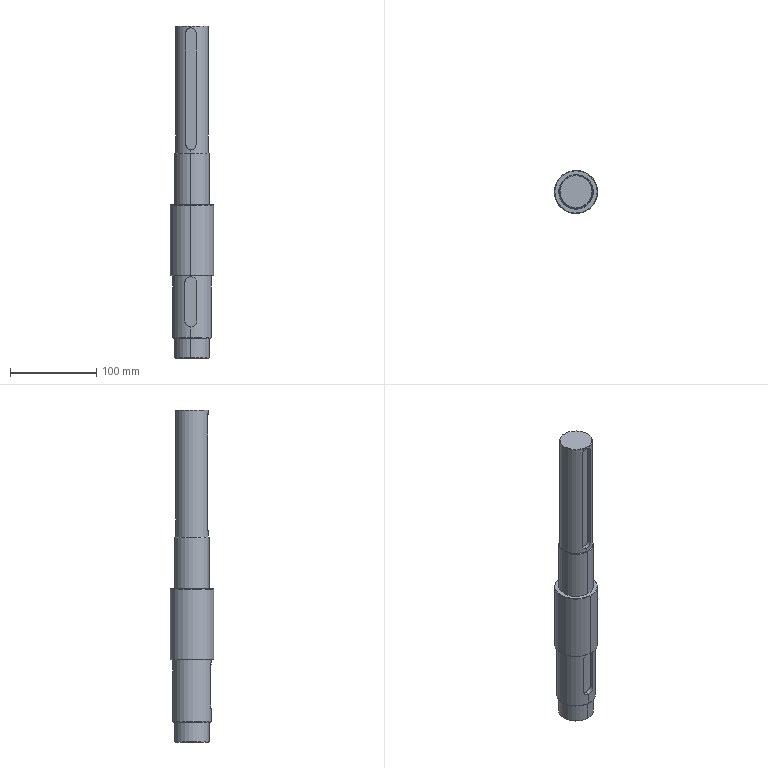Part | SolidWorks | features BaseBody 1 | 1 solid | 40 faces | box 50 x 50 x 384 mm | volume 534684 mm3 | cylinder 16 | cone 12 | plane 12 | commonest cylinder face diameters 40 x4 12 x3 14 x3 38 x2 45 x2 50 x2
STEP:
#1=CARTESIAN_POINT('',(581.983,5.282,-315.693));
#2=VERTEX_POINT('',#1);
#3=CARTESIAN_POINT('',(575.002,5.788,-322.693));
#4=VERTEX_POINT('',#3);
#5=CARTESIAN_POINT('',(575.002,5.788,-315.693));
#6=DIRECTION('',(0.07229,0.9974,0.));
#7=DIRECTION('',(0.,0.,1.));
#8=AXIS2_PLACEMENT_3D('',#5,#6,#7);
#9=CIRCLE('',#8,7.);
#10=EDGE_CURVE('',#2,#4,#9,.T.);
#11=ORIENTED_EDGE('',*,*,#10,.T.);
#12=CARTESIAN_POINT('',(574.604,0.3028,-322.693));
#13=VERTEX_POINT('',#12);
#14=CARTESIAN_POINT('',(575.002,5.788,-322.693));
#15=DIRECTION('',(-0.07229,-0.9974,0.));
#16=VECTOR('',#15,1000.);
#17=LINE('',#14,#16);
#18=EDGE_CURVE('',#4,#13,#17,.T.);
#19=ORIENTED_EDGE('',*,*,#18,.T.);
#20=CARTESIAN_POINT('',(581.667,0.9105,-315.693));
#21=VERTEX_POINT('',#20);
#22=CARTESIAN_POINT('',(574.604,0.3028,-322.693));
#23=CARTESIAN_POINT('',(575.062,0.2696,-322.693));
#24=CARTESIAN_POINT('',(575.529,0.2504,-322.647));
#25=CARTESIAN_POINT('',(576.43,0.2403,-322.466));
#26=CARTESIAN_POINT('',(576.869,0.2489,-322.333));
#27=CARTESIAN_POINT('',(577.511,0.2794,-322.068));
#28=CARTESIAN_POINT('',(577.721,0.2925,-321.969));
#29=CARTESIAN_POINT('',(578.127,0.3231,-321.753));
#30=CARTESIAN_POINT('',(578.323,0.3407,-321.635));
#31=CARTESIAN_POINT('',(578.704,0.3795,-321.383));
#32=CARTESIAN_POINT('',(578.889,0.4008,-321.247));
#33=CARTESIAN_POINT('',(579.245,0.4461,-320.958));
#34=CARTESIAN_POINT('',(579.418,0.4703,-320.803));
#35=CARTESIAN_POINT('',(579.909,0.5442,-320.319));
#36=CARTESIAN_POINT('',(580.201,0.5954,-319.969));
#37=CARTESIAN_POINT('',(580.715,0.6939,-319.214));
#38=CARTESIAN_POINT('',(580.939,0.7414,-318.805));
#39=CARTESIAN_POINT('',(581.297,0.8209,-317.963));
#40=CARTESIAN_POINT('',(581.433,0.8535,-317.527));
#41=CARTESIAN_POINT('',(581.572,0.8872,-316.849));
#42=CARTESIAN_POINT('',(581.608,0.8959,-316.619));
#43=CARTESIAN_POINT('',(581.655,0.9075,-316.157));
#44=CARTESIAN_POINT('',(581.667,0.9105,-315.926));
#45=CARTESIAN_POINT('',(581.667,0.9105,-315.693));
#46=B_SPLINE_CURVE_WITH_KNOTS('',3,(#22,#23,#24,#25,#26,#27,#28,#29,#30,#31,#32,#33,#34,#35,#36,#37,#38,#39,#40,#41,#42,#43,#44,#45),.UNSPECIFIED.,.F.,.F.,(4,2,2,2,2,2,2,2,2,2,2,4),(0.01101,0.01239,0.01376,0.01445,0.01514,0.01583,0.01651,0.01789,0.01926,0.02064,0.02133,0.02201),.UNSPECIFIED.);
#47=EDGE_CURVE('',#13,#21,#46,.T.);
#48=ORIENTED_EDGE('',*,*,#47,.T.);
#49=CARTESIAN_POINT('',(581.983,5.282,-315.693));
#50=DIRECTION('',(-0.07229,-0.9974,0.));
#51=VECTOR('',#50,1000.);
#52=LINE('',#49,#51);
#53=EDGE_CURVE('',#2,#21,#52,.T.);
#54=ORIENTED_EDGE('',*,*,#53,.F.);
#55=EDGE_LOOP('',(#11,#19,#48,#54));
#56=FACE_OUTER_BOUND('',#55,.T.);
#57=CARTESIAN_POINT('',(575.002,5.788,-315.693));
#58=DIRECTION('',(-0.07229,-0.9974,0.));
#59=DIRECTION('',(0.,0.,-1.));
#60=AXIS2_PLACEMENT_3D('',#57,#58,#59);
#61=CYLINDRICAL_SURFACE('',#60,7.);
#62=ADVANCED_FACE('',(#56),#61,.F.);
#63=CARTESIAN_POINT('',(574.893,4.292,25.307));
#64=VERTEX_POINT('',#63);
#65=CARTESIAN_POINT('',(577.568,41.196,25.307));
#66=VERTEX_POINT('',#65);
#67=CARTESIAN_POINT('',(576.231,22.744,25.307));
#68=DIRECTION('',(0.,0.,1.));
#69=DIRECTION('',(-0.07229,-0.9974,0.));
#70=AXIS2_PLACEMENT_3D('',#67,#68,#69);
#71=CIRCLE('',#70,18.5);
#72=EDGE_CURVE('',#64,#66,#71,.T.);
#73=ORIENTED_EDGE('',*,*,#72,.F.);
#74=CARTESIAN_POINT('',(574.857,3.794,24.807));
#75=VERTEX_POINT('',#74);
#76=CARTESIAN_POINT('',(574.893,4.292,25.307));
#77=DIRECTION('',(-0.05112,-0.7053,-0.7071));
#78=VECTOR('',#77,1000.);
#79=LINE('',#76,#78);
#80=EDGE_CURVE('',#64,#75,#79,.T.);
#81=ORIENTED_EDGE('',*,*,#80,.T.);
#82=CARTESIAN_POINT('',(577.604,41.694,24.807));
#83=VERTEX_POINT('',#82);
#84=CARTESIAN_POINT('',(576.231,22.744,24.807));
#85=DIRECTION('',(0.,0.,-1.));
#86=DIRECTION('',(-0.07229,-0.9974,0.));
#87=AXIS2_PLACEMENT_3D('',#84,#85,#86);
#88=CIRCLE('',#87,19.);
#89=EDGE_CURVE('',#83,#75,#88,.T.);
#90=ORIENTED_EDGE('',*,*,#89,.F.);
#91=CARTESIAN_POINT('',(577.568,41.196,25.307));
#92=DIRECTION('',(0.05112,0.7053,-0.7071));
#93=VECTOR('',#92,1000.);
#94=LINE('',#91,#93);
#95=EDGE_CURVE('',#66,#83,#94,.T.);
#96=ORIENTED_EDGE('',*,*,#95,.F.);
#97=EDGE_LOOP('',(#73,#81,#90,#96));
#98=FACE_OUTER_BOUND('',#97,.T.);
#99=CARTESIAN_POINT('',(576.231,22.744,25.307));
#100=DIRECTION('',(0.,0.,-1.));
#101=DIRECTION('',(0.07229,0.9974,0.));
#102=AXIS2_PLACEMENT_3D('',#99,#100,#101);
#103=CONICAL_SURFACE('',#102,18.5,0.7854);
#104=ADVANCED_FACE('',(#98),#103,.T.);
#105=CARTESIAN_POINT('',(577.64,42.193,-358.693));
#106=VERTEX_POINT('',#105);
#107=CARTESIAN_POINT('',(574.821,3.295,-358.693));
#108=VERTEX_POINT('',#107);
#109=CARTESIAN_POINT('',(576.231,22.744,-358.693));
#110=DIRECTION('',(0.,0.,-1.));
#111=DIRECTION('',(0.07229,0.9974,0.));
#112=AXIS2_PLACEMENT_3D('',#109,#110,#111);
#113=CIRCLE('',#112,19.5);
#114=EDGE_CURVE('',#106,#108,#113,.T.);
#115=ORIENTED_EDGE('',*,*,#114,.F.);
#116=CARTESIAN_POINT('',(577.676,42.692,-358.193));
#117=VERTEX_POINT('',#116);
#118=CARTESIAN_POINT('',(577.64,42.193,-358.693));
#119=DIRECTION('',(0.05112,0.7053,0.7071));
#120=VECTOR('',#119,1000.);
#121=LINE('',#118,#120);
#122=EDGE_CURVE('',#106,#117,#121,.T.);
#123=ORIENTED_EDGE('',*,*,#122,.T.);
#124=CARTESIAN_POINT('',(574.785,2.796,-358.193));
#125=VERTEX_POINT('',#124);
#126=CARTESIAN_POINT('',(576.231,22.744,-358.193));
#127=DIRECTION('',(0.,0.,1.));
#128=DIRECTION('',(0.07229,0.9974,0.));
#129=AXIS2_PLACEMENT_3D('',#126,#127,#128);
#130=CIRCLE('',#129,20.);
#131=EDGE_CURVE('',#125,#117,#130,.T.);
#132=ORIENTED_EDGE('',*,*,#131,.F.);
#133=CARTESIAN_POINT('',(574.821,3.295,-358.693));
#134=DIRECTION('',(-0.05112,-0.7053,0.7071));
#135=VECTOR('',#134,1000.);
#136=LINE('',#133,#135);
#137=EDGE_CURVE('',#108,#125,#136,.T.);
#138=ORIENTED_EDGE('',*,*,#137,.F.);
#139=EDGE_LOOP('',(#115,#123,#132,#138));
#140=FACE_OUTER_BOUND('',#139,.T.);
#141=CARTESIAN_POINT('',(576.231,22.744,-358.693));
#142=DIRECTION('',(0.,0.,1.));
#143=DIRECTION('',(-0.07229,-0.9974,0.));
#144=AXIS2_PLACEMENT_3D('',#141,#142,#143);
#145=CONICAL_SURFACE('',#144,19.5,0.7854);
#146=ADVANCED_FACE('',(#140),#145,.T.);
#147=CARTESIAN_POINT('',(577.821,44.686,-335.693));
#148=VERTEX_POINT('',#147);
#149=CARTESIAN_POINT('',(574.64,0.8015,-335.693));
#150=VERTEX_POINT('',#149);
#151=CARTESIAN_POINT('',(576.231,22.744,-335.693));
#152=DIRECTION('',(0.,0.,-1.));
#153=DIRECTION('',(0.07229,0.9974,0.));
#154=AXIS2_PLACEMENT_3D('',#151,#152,#153);
#155=CIRCLE('',#154,22.);
#156=EDGE_CURVE('',#148,#150,#155,.T.);
#157=ORIENTED_EDGE('',*,*,#156,.F.);
#158=CARTESIAN_POINT('',(577.857,45.185,-335.193));
#159=VERTEX_POINT('',#158);
#160=CARTESIAN_POINT('',(577.821,44.686,-335.693));
#161=DIRECTION('',(0.05112,0.7053,0.7071));
#162=VECTOR('',#161,1000.);
#163=LINE('',#160,#162);
#164=EDGE_CURVE('',#148,#159,#163,.T.);
#165=ORIENTED_EDGE('',*,*,#164,.T.);
#166=CARTESIAN_POINT('',(574.604,0.3028,-335.193));
#167=VERTEX_POINT('',#166);
#168=CARTESIAN_POINT('',(576.231,22.744,-335.193));
#169=DIRECTION('',(0.,0.,1.));
#170=DIRECTION('',(0.07229,0.9974,0.));
#171=AXIS2_PLACEMENT_3D('',#168,#169,#170);
#172=CIRCLE('',#171,22.5);
#173=EDGE_CURVE('',#167,#159,#172,.T.);
#174=ORIENTED_EDGE('',*,*,#173,.F.);
#175=CARTESIAN_POINT('',(574.64,0.8015,-335.693));
#176=DIRECTION('',(-0.05112,-0.7053,0.7071));
#177=VECTOR('',#176,1000.);
#178=LINE('',#175,#177);
#179=EDGE_CURVE('',#150,#167,#178,.T.);
#180=ORIENTED_EDGE('',*,*,#179,.F.);
#181=EDGE_LOOP('',(#157,#165,#174,#180));
#182=FACE_OUTER_BOUND('',#181,.T.);
#183=CARTESIAN_POINT('',(576.231,22.744,-335.693));
#184=DIRECTION('',(0.,0.,1.));
#185=DIRECTION('',(-0.07229,-0.9974,0.));
#186=AXIS2_PLACEMENT_3D('',#183,#184,#185);
#187=CONICAL_SURFACE('',#186,22.,0.7854);
#188=ADVANCED_FACE('',(#182),#187,.T.);
#189=CARTESIAN_POINT('',(578.002,47.18,-263.693));
#190=VERTEX_POINT('',#189);
#191=CARTESIAN_POINT('',(574.46,-1.692,-263.693));
#192=VERTEX_POINT('',#191);
#193=CARTESIAN_POINT('',(576.231,22.744,-263.693));
#194=DIRECTION('',(0.,0.,-1.));
#195=DIRECTION('',(0.07229,0.9974,0.));
#196=AXIS2_PLACEMENT_3D('',#193,#194,#195);
#197=CIRCLE('',#196,24.5);
#198=EDGE_CURVE('',#190,#192,#197,.T.);
#199=ORIENTED_EDGE('',*,*,#198,.F.);
#200=CARTESIAN_POINT('',(578.038,47.679,-263.193));
#201=VERTEX_POINT('',#200);
#202=CARTESIAN_POINT('',(578.002,47.18,-263.693));
#203=DIRECTION('',(0.05112,0.7053,0.7071));
#204=VECTOR('',#203,1000.);
#205=LINE('',#202,#204);
#206=EDGE_CURVE('',#190,#201,#205,.T.);
#207=ORIENTED_EDGE('',*,*,#206,.T.);
#208=CARTESIAN_POINT('',(574.423,-2.191,-263.193));
#209=VERTEX_POINT('',#208);
#210=CARTESIAN_POINT('',(576.231,22.744,-263.193));
#211=DIRECTION('',(0.,0.,1.));
#212=DIRECTION('',(0.07229,0.9974,0.));
#213=AXIS2_PLACEMENT_3D('',#210,#211,#212);
#214=CIRCLE('',#213,25.);
#215=EDGE_CURVE('',#209,#201,#214,.T.);
#216=ORIENTED_EDGE('',*,*,#215,.F.);
#217=CARTESIAN_POINT('',(574.46,-1.692,-263.693));
#218=DIRECTION('',(-0.05112,-0.7053,0.7071));
#219=VECTOR('',#218,1000.);
#220=LINE('',#217,#219);
#221=EDGE_CURVE('',#192,#209,#220,.T.);
#222=ORIENTED_EDGE('',*,*,#221,.F.);
#223=EDGE_LOOP('',(#199,#207,#216,#222));
#224=FACE_OUTER_BOUND('',#223,.T.);
#225=CARTESIAN_POINT('',(576.231,22.744,-263.693));
#226=DIRECTION('',(0.,0.,1.));
#227=DIRECTION('',(-0.07229,-0.9974,0.));
#228=AXIS2_PLACEMENT_3D('',#225,#226,#227);
#229=CONICAL_SURFACE('',#228,24.5,0.7854);
#230=ADVANCED_FACE('',(#224),#229,.T.);
#231=CARTESIAN_POINT('',(574.821,3.295,-121.693));
#232=VERTEX_POINT('',#231);
#233=CARTESIAN_POINT('',(577.64,42.193,-121.693));
#234=VERTEX_POINT('',#233);
#235=CARTESIAN_POINT('',(576.231,22.744,-121.693));
#236=DIRECTION('',(0.,0.,1.));
#237=DIRECTION('',(-0.07229,-0.9974,0.));
#238=AXIS2_PLACEMENT_3D('',#235,#236,#237);
#239=CIRCLE('',#238,19.5);
#240=EDGE_CURVE('',#232,#234,#239,.T.);
#241=ORIENTED_EDGE('',*,*,#240,.F.);
#242=CARTESIAN_POINT('',(574.785,2.796,-122.193));
#243=VERTEX_POINT('',#242);
#244=CARTESIAN_POINT('',(574.821,3.295,-121.693));
#245=DIRECTION('',(-0.05112,-0.7053,-0.7071));
#246=VECTOR('',#245,1000.);
#247=LINE('',#244,#246);
#248=EDGE_CURVE('',#232,#243,#247,.T.);
#249=ORIENTED_EDGE('',*,*,#248,.T.);
#250=CARTESIAN_POINT('',(577.676,42.692,-122.193));
#251=VERTEX_POINT('',#250);
#252=CARTESIAN_POINT('',(576.231,22.744,-122.193));
#253=DIRECTION('',(0.,0.,-1.));
#254=DIRECTION('',(-0.07229,-0.9974,0.));
#255=AXIS2_PLACEMENT_3D('',#252,#253,#254);
#256=CIRCLE('',#255,20.);
#257=EDGE_CURVE('',#251,#243,#256,.T.);
#258=ORIENTED_EDGE('',*,*,#257,.F.);
#259=CARTESIAN_POINT('',(577.64,42.193,-121.693));
#260=DIRECTION('',(0.05112,0.7053,-0.7071));
#261=VECTOR('',#260,1000.);
#262=LINE('',#259,#261);
#263=EDGE_CURVE('',#234,#251,#262,.T.);
#264=ORIENTED_EDGE('',*,*,#263,.F.);
#265=EDGE_LOOP('',(#241,#249,#258,#264));
#266=FACE_OUTER_BOUND('',#265,.T.);
#267=CARTESIAN_POINT('',(576.231,22.744,-121.693));
#268=DIRECTION('',(0.,0.,-1.));
#269=DIRECTION('',(0.07229,0.9974,0.));
#270=AXIS2_PLACEMENT_3D('',#267,#268,#269);
#271=CONICAL_SURFACE('',#270,19.5,0.7854);
#272=ADVANCED_FACE('',(#266),#271,.T.);
#273=CARTESIAN_POINT('',(574.46,-1.692,-181.693));
#274=VERTEX_POINT('',#273);
#275=CARTESIAN_POINT('',(578.002,47.18,-181.693));
#276=VERTEX_POINT('',#275);
#277=CARTESIAN_POINT('',(576.231,22.744,-181.693));
#278=DIRECTION('',(0.,0.,1.));
#279=DIRECTION('',(0.07229,0.9974,0.));
#280=AXIS2_PLACEMENT_3D('',#277,#278,#279);
#281=CIRCLE('',#280,24.5);
#282=EDGE_CURVE('',#274,#276,#281,.T.);
#283=ORIENTED_EDGE('',*,*,#282,.F.);
#284=CARTESIAN_POINT('',(574.423,-2.191,-182.193));
#285=VERTEX_POINT('',#284);
#286=CARTESIAN_POINT('',(574.423,-2.191,-182.193));
#287=DIRECTION('',(-0.05112,-0.7053,-0.7071));
#288=VECTOR('',#287,1000.);
#289=LINE('',#286,#288);
#290=EDGE_CURVE('',#274,#285,#289,.T.);
#291=ORIENTED_EDGE('',*,*,#290,.T.);
#292=CARTESIAN_POINT('',(578.038,47.679,-182.193));
#293=VERTEX_POINT('',#292);
#294=CARTESIAN_POINT('',(576.231,22.744,-182.193));
#295=DIRECTION('',(0.,0.,-1.));
#296=DIRECTION('',(0.07229,0.9974,0.));
#297=AXIS2_PLACEMENT_3D('',#294,#295,#296);
#298=CIRCLE('',#297,25.);
#299=EDGE_CURVE('',#293,#285,#298,.T.);
#300=ORIENTED_EDGE('',*,*,#299,.F.);
#301=CARTESIAN_POINT('',(578.038,47.679,-182.193));
#302=DIRECTION('',(0.05112,0.7053,-0.7071));
#303=VECTOR('',#302,1000.);
#304=LINE('',#301,#303);
#305=EDGE_CURVE('',#276,#293,#304,.T.);
#306=ORIENTED_EDGE('',*,*,#305,.F.);
#307=EDGE_LOOP('',(#283,#291,#300,#306));
#308=FACE_OUTER_BOUND('',#307,.T.);
#309=CARTESIAN_POINT('',(576.231,22.744,-182.193));
#310=DIRECTION('',(0.,0.,-1.));
#311=DIRECTION('',(0.07229,0.9974,0.));
#312=AXIS2_PLACEMENT_3D('',#309,#310,#311);
#313=CONICAL_SURFACE('',#312,25.,0.7854);
#314=ADVANCED_FACE('',(#308),#313,.T.);
#315=CARTESIAN_POINT('',(581.203,8.347,-111.693));
#316=VERTEX_POINT('',#315);
#317=CARTESIAN_POINT('',(575.219,8.781,-117.693));
#318=VERTEX_POINT('',#317);
#319=CARTESIAN_POINT('',(575.219,8.781,-111.693));
#320=DIRECTION('',(0.07229,0.9974,0.));
#321=DIRECTION('',(0.,0.,1.));
#322=AXIS2_PLACEMENT_3D('',#319,#320,#321);
#323=CIRCLE('',#322,6.);
#324=EDGE_CURVE('',#316,#318,#323,.T.);
#325=ORIENTED_EDGE('',*,*,#324,.T.);
#326=CARTESIAN_POINT('',(574.857,3.794,-117.693));
#327=VERTEX_POINT('',#326);
#328=CARTESIAN_POINT('',(575.219,8.781,-117.693));
#329=DIRECTION('',(-0.07229,-0.9974,0.));
#330=VECTOR('',#329,1000.);
#331=LINE('',#328,#330);
#332=EDGE_CURVE('',#318,#327,#331,.T.);
#333=ORIENTED_EDGE('',*,*,#332,.T.);
#334=CARTESIAN_POINT('',(580.912,4.33,-111.693));
#335=VERTEX_POINT('',#334);
#336=CARTESIAN_POINT('',(574.857,3.794,-117.693));
#337=CARTESIAN_POINT('',(575.25,3.765,-117.693));
#338=CARTESIAN_POINT('',(575.65,3.749,-117.653));
#339=CARTESIAN_POINT('',(576.422,3.741,-117.499));
#340=CARTESIAN_POINT('',(576.799,3.749,-117.384));
#341=CARTESIAN_POINT('',(577.533,3.785,-117.081));
#342=CARTESIAN_POINT('',(577.882,3.813,-116.895));
#343=CARTESIAN_POINT('',(578.372,3.864,-116.57));
#344=CARTESIAN_POINT('',(578.53,3.883,-116.454));
#345=CARTESIAN_POINT('',(578.836,3.923,-116.206));
#346=CARTESIAN_POINT('',(578.984,3.944,-116.073));
#347=CARTESIAN_POINT('',(579.404,4.009,-115.658));
#348=CARTESIAN_POINT('',(579.655,4.054,-115.358));
#349=CARTESIAN_POINT('',(580.096,4.14,-114.711));
#350=CARTESIAN_POINT('',(580.288,4.182,-114.361));
#351=CARTESIAN_POINT('',(580.594,4.251,-113.639));
#352=CARTESIAN_POINT('',(580.711,4.28,-113.265));
#353=CARTESIAN_POINT('',(580.871,4.319,-112.49));
#354=CARTESIAN_POINT('',(580.912,4.33,-112.092));
#355=CARTESIAN_POINT('',(580.912,4.33,-111.693));
#356=B_SPLINE_CURVE_WITH_KNOTS('',3,(#336,#337,#338,#339,#340,#341,#342,#343,#344,#345,#346,#347,#348,#349,#350,#351,#352,#353,#354,#355),.UNSPECIFIED.,.F.,.F.,(4,2,2,2,2,2,2,2,2,4),(0.009443,0.01062,0.0118,0.01298,0.01357,0.01416,0.01534,0.01652,0.01769,0.01887),.UNSPECIFIED.);
#357=EDGE_CURVE('',#327,#335,#356,.T.);
#358=ORIENTED_EDGE('',*,*,#357,.T.);
#359=CARTESIAN_POINT('',(581.203,8.347,-111.693));
#360=DIRECTION('',(-0.07229,-0.9974,0.));
#361=VECTOR('',#360,1000.);
#362=LINE('',#359,#361);
#363=EDGE_CURVE('',#316,#335,#362,.T.);
#364=ORIENTED_EDGE('',*,*,#363,.F.);
#365=EDGE_LOOP('',(#325,#333,#358,#364));
#366=FACE_OUTER_BOUND('',#365,.T.);
#367=CARTESIAN_POINT('',(575.219,8.781,-111.693));
#368=DIRECTION('',(-0.07229,-0.9974,0.));
#369=DIRECTION('',(0.,0.,-1.));
#370=AXIS2_PLACEMENT_3D('',#367,#368,#369);
#371=CYLINDRICAL_SURFACE('',#370,6.);
#372=ADVANCED_FACE('',(#366),#371,.F.);
#373=ORIENTED_EDGE('',*,*,#257,.T.);
#374=CARTESIAN_POINT('',(574.785,2.796,-181.693));
#375=VERTEX_POINT('',#374);
#376=CARTESIAN_POINT('',(574.785,2.796,-121.693));
#377=DIRECTION('',(0.,0.,-1.));
#378=VECTOR('',#377,1000.);
#379=LINE('',#376,#378);
#380=EDGE_CURVE('',#243,#375,#379,.T.);
#381=ORIENTED_EDGE('',*,*,#380,.T.);
#382=CARTESIAN_POINT('',(577.676,42.692,-181.693));
#383=VERTEX_POINT('',#382);
#384=CARTESIAN_POINT('',(576.231,22.744,-181.693));
#385=DIRECTION('',(0.,0.,1.));
#386=DIRECTION('',(0.07229,0.9974,0.));
#387=AXIS2_PLACEMENT_3D('',#384,#385,#386);
#388=CIRCLE('',#387,20.);
#389=EDGE_CURVE('',#375,#383,#388,.T.);
#390=ORIENTED_EDGE('',*,*,#389,.T.);
#391=CARTESIAN_POINT('',(577.676,42.692,-121.693));
#392=DIRECTION('',(0.,0.,-1.));
#393=VECTOR('',#392,1000.);
#394=LINE('',#391,#393);
#395=EDGE_CURVE('',#251,#383,#394,.T.);
#396=ORIENTED_EDGE('',*,*,#395,.F.);
#397=EDGE_LOOP('',(#373,#381,#390,#396));
#398=FACE_OUTER_BOUND('',#397,.T.);
#399=CARTESIAN_POINT('',(576.231,22.744,-121.693));
#400=DIRECTION('',(0.,0.,-1.));
#401=DIRECTION('',(0.07229,0.9974,0.));
#402=AXIS2_PLACEMENT_3D('',#399,#400,#401);
#403=CYLINDRICAL_SURFACE('',#402,20.);
#404=ADVANCED_FACE('',(#398),#403,.T.);
#405=ORIENTED_EDGE('',*,*,#131,.T.);
#406=CARTESIAN_POINT('',(577.676,42.692,-335.693));
#407=VERTEX_POINT('',#406);
#408=CARTESIAN_POINT('',(577.676,42.692,-358.693));
#409=DIRECTION('',(0.,0.,1.));
#410=VECTOR('',#409,1000.);
#411=LINE('',#408,#410);
#412=EDGE_CURVE('',#117,#407,#411,.T.);
#413=ORIENTED_EDGE('',*,*,#412,.T.);
#414=CARTESIAN_POINT('',(574.785,2.796,-335.693));
#415=VERTEX_POINT('',#414);
#416=CARTESIAN_POINT('',(576.231,22.744,-335.693));
#417=DIRECTION('',(0.,0.,-1.));
#418=DIRECTION('',(0.07229,0.9974,0.));
#419=AXIS2_PLACEMENT_3D('',#416,#417,#418);
#420=CIRCLE('',#419,20.);
#421=EDGE_CURVE('',#407,#415,#420,.T.);
#422=ORIENTED_EDGE('',*,*,#421,.T.);
#423=CARTESIAN_POINT('',(574.785,2.796,-358.693));
#424=DIRECTION('',(0.,0.,1.));
#425=VECTOR('',#424,1000.);
#426=LINE('',#423,#425);
#427=EDGE_CURVE('',#125,#415,#426,.T.);
#428=ORIENTED_EDGE('',*,*,#427,.F.);
#429=EDGE_LOOP('',(#405,#413,#422,#428));
#430=FACE_OUTER_BOUND('',#429,.T.);
#431=CARTESIAN_POINT('',(576.231,22.744,-358.693));
#432=DIRECTION('',(0.,0.,1.));
#433=DIRECTION('',(-0.07229,-0.9974,0.));
#434=AXIS2_PLACEMENT_3D('',#431,#432,#433);
#435=CYLINDRICAL_SURFACE('',#434,20.);
#436=ADVANCED_FACE('',(#430),#435,.T.);
#437=ORIENTED_EDGE('',*,*,#215,.T.);
#438=CARTESIAN_POINT('',(578.038,47.679,-263.693));
#439=DIRECTION('',(0.,0.,1.));
#440=VECTOR('',#439,1000.);
#441=LINE('',#438,#440);
#442=EDGE_CURVE('',#201,#293,#441,.T.);
#443=ORIENTED_EDGE('',*,*,#442,.T.);
#444=ORIENTED_EDGE('',*,*,#299,.T.);
#445=CARTESIAN_POINT('',(574.423,-2.191,-263.693));
#446=DIRECTION('',(0.,0.,1.));
#447=VECTOR('',#446,1000.);
#448=LINE('',#445,#447);
#449=EDGE_CURVE('',#209,#285,#448,.T.);
#450=ORIENTED_EDGE('',*,*,#449,.F.);
#451=EDGE_LOOP('',(#437,#443,#444,#450));
#452=FACE_OUTER_BOUND('',#451,.T.);
#453=CARTESIAN_POINT('',(576.231,22.744,-263.693));
#454=DIRECTION('',(0.,0.,1.));
#455=DIRECTION('',(-0.07229,-0.9974,0.));
#456=AXIS2_PLACEMENT_3D('',#453,#454,#455);
#457=CYLINDRICAL_SURFACE('',#456,25.);
#458=ADVANCED_FACE('',(#452),#457,.T.);
#459=ORIENTED_EDGE('',*,*,#89,.T.);
#460=CARTESIAN_POINT('',(574.857,3.794,23.307));
#461=VERTEX_POINT('',#460);
#462=CARTESIAN_POINT('',(574.857,3.794,25.307));
#463=DIRECTION('',(0.,0.,-1.));
#464=VECTOR('',#463,1000.);
#465=LINE('',#462,#464);
#466=EDGE_CURVE('',#75,#461,#465,.T.);
#467=ORIENTED_EDGE('',*,*,#466,.T.);
#468=CARTESIAN_POINT('',(580.912,4.33,17.307));
#469=VERTEX_POINT('',#468);
#470=CARTESIAN_POINT('',(580.912,4.33,17.307));
#471=CARTESIAN_POINT('',(580.912,4.33,17.706));
#472=CARTESIAN_POINT('',(580.871,4.319,18.098));
#473=CARTESIAN_POINT('',(580.753,4.29,18.676));
#474=CARTESIAN_POINT('',(580.704,4.278,18.867));
#475=CARTESIAN_POINT('',(580.587,4.25,19.246));
#476=CARTESIAN_POINT('',(580.518,4.234,19.433));
#477=CARTESIAN_POINT('',(580.287,4.181,19.977));
#478=CARTESIAN_POINT('',(580.099,4.141,20.321));
#479=CARTESIAN_POINT('',(579.767,4.076,20.808));
#480=CARTESIAN_POINT('',(579.647,4.053,20.967));
#481=CARTESIAN_POINT('',(579.394,4.009,21.27));
#482=CARTESIAN_POINT('',(579.261,3.987,21.414));
#483=CARTESIAN_POINT('',(578.843,3.922,21.826));
#484=CARTESIAN_POINT('',(578.538,3.882,22.074));
#485=CARTESIAN_POINT('',(577.876,3.812,22.513));
#486=CARTESIAN_POINT('',(577.528,3.785,22.697));
#487=CARTESIAN_POINT('',(576.983,3.758,22.922));
#488=CARTESIAN_POINT('',(576.798,3.751,22.989));
#489=CARTESIAN_POINT('',(576.419,3.744,23.104));
#490=CARTESIAN_POINT('',(576.225,3.743,23.152));
#491=CARTESIAN_POINT('',(575.642,3.749,23.269));
#492=CARTESIAN_POINT('',(575.251,3.765,23.307));
#493=CARTESIAN_POINT('',(574.857,3.794,23.307));
#494=B_SPLINE_CURVE_WITH_KNOTS('',3,(#470,#471,#472,#473,#474,#475,#476,#477,#478,#479,#480,#481,#482,#483,#484,#485,#486,#487,#488,#489,#490,#491,#492,#493),.UNSPECIFIED.,.F.,.F.,(4,2,2,2,2,2,2,2,2,2,2,4),(0.,0.00118,0.00177,0.002361,0.003541,0.004131,0.004721,0.005902,0.007082,0.007672,0.008262,0.009443),.UNSPECIFIED.);
#495=EDGE_CURVE('',#469,#461,#494,.T.);
#496=ORIENTED_EDGE('',*,*,#495,.F.);
#497=CARTESIAN_POINT('',(580.912,4.33,25.307));
#498=DIRECTION('',(0.,0.,1.));
#499=VECTOR('',#498,1000.);
#500=LINE('',#497,#499);
#501=EDGE_CURVE('',#335,#469,#500,.T.);
#502=ORIENTED_EDGE('',*,*,#501,.F.);
#503=ORIENTED_EDGE('',*,*,#357,.F.);
#504=CARTESIAN_POINT('',(574.857,3.794,-121.693));
#505=VERTEX_POINT('',#504);
#506=CARTESIAN_POINT('',(574.857,3.794,25.307));
#507=DIRECTION('',(0.,0.,-1.));
#508=VECTOR('',#507,1000.);
#509=LINE('',#506,#508);
#510=EDGE_CURVE('',#327,#505,#509,.T.);
#511=ORIENTED_EDGE('',*,*,#510,.T.);
#512=CARTESIAN_POINT('',(577.604,41.694,-121.693));
#513=VERTEX_POINT('',#512);
#514=CARTESIAN_POINT('',(576.231,22.744,-121.693));
#515=DIRECTION('',(0.,0.,1.));
#516=DIRECTION('',(-0.07229,-0.9974,0.));
#517=AXIS2_PLACEMENT_3D('',#514,#515,#516);
#518=CIRCLE('',#517,19.);
#519=EDGE_CURVE('',#505,#513,#518,.T.);
#520=ORIENTED_EDGE('',*,*,#519,.T.);
#521=CARTESIAN_POINT('',(577.604,41.694,25.307));
#522=DIRECTION('',(0.,0.,-1.));
#523=VECTOR('',#522,1000.);
#524=LINE('',#521,#523);
#525=EDGE_CURVE('',#83,#513,#524,.T.);
#526=ORIENTED_EDGE('',*,*,#525,.F.);
#527=EDGE_LOOP('',(#459,#467,#496,#502,#503,#511,#520,#526));
#528=FACE_OUTER_BOUND('',#527,.T.);
#529=CARTESIAN_POINT('',(576.231,22.744,25.307));
#530=DIRECTION('',(0.,0.,-1.));
#531=DIRECTION('',(0.07229,0.9974,0.));
#532=AXIS2_PLACEMENT_3D('',#529,#530,#531);
#533=CYLINDRICAL_SURFACE('',#532,19.);
#534=ADVANCED_FACE('',(#528),#533,.T.);
#535=ORIENTED_EDGE('',*,*,#173,.T.);
#536=CARTESIAN_POINT('',(577.857,45.185,-263.693));
#537=VERTEX_POINT('',#536);
#538=CARTESIAN_POINT('',(577.857,45.185,-335.693));
#539=DIRECTION('',(0.,0.,1.));
#540=VECTOR('',#539,1000.);
#541=LINE('',#538,#540);
#542=EDGE_CURVE('',#159,#537,#541,.T.);
#543=ORIENTED_EDGE('',*,*,#542,.T.);
#544=CARTESIAN_POINT('',(574.604,0.3028,-263.693));
#545=VERTEX_POINT('',#544);
#546=CARTESIAN_POINT('',(576.231,22.744,-263.693));
#547=DIRECTION('',(0.,0.,-1.));
#548=DIRECTION('',(0.07229,0.9974,0.));
#549=AXIS2_PLACEMENT_3D('',#546,#547,#548);
#550=CIRCLE('',#549,22.5);
#551=EDGE_CURVE('',#537,#545,#550,.T.);
#552=ORIENTED_EDGE('',*,*,#551,.T.);
#553=CARTESIAN_POINT('',(574.604,0.3028,-264.693));
#554=VERTEX_POINT('',#553);
#555=CARTESIAN_POINT('',(574.604,0.3028,-335.693));
#556=DIRECTION('',(0.,0.,1.));
#557=VECTOR('',#556,1000.);
#558=LINE('',#555,#557);
#559=EDGE_CURVE('',#554,#545,#558,.T.);
#560=ORIENTED_EDGE('',*,*,#559,.F.);
#561=CARTESIAN_POINT('',(581.667,0.9105,-271.693));
#562=VERTEX_POINT('',#561);
#563=CARTESIAN_POINT('',(581.667,0.9105,-271.693));
#564=CARTESIAN_POINT('',(581.667,0.9105,-271.227));
#565=CARTESIAN_POINT('',(581.62,0.8986,-270.77));
#566=CARTESIAN_POINT('',(581.482,0.8653,-270.096));
#567=CARTESIAN_POINT('',(581.425,0.8516,-269.873));
#568=CARTESIAN_POINT('',(581.288,0.8195,-269.432));
#569=CARTESIAN_POINT('',(581.207,0.8011,-269.213));
#570=CARTESIAN_POINT('',(580.938,0.7411,-268.578));
#571=CARTESIAN_POINT('',(580.719,0.6946,-268.177));
#572=CARTESIAN_POINT('',(580.331,0.6204,-267.608));
#573=CARTESIAN_POINT('',(580.191,0.5948,-267.423));
#574=CARTESIAN_POINT('',(579.896,0.5441,-267.07));
#575=CARTESIAN_POINT('',(579.741,0.5189,-266.901));
#576=CARTESIAN_POINT('',(579.253,0.4455,-266.421));
#577=CARTESIAN_POINT('',(578.898,0.3993,-266.132));
#578=CARTESIAN_POINT('',(578.126,0.3205,-265.62));
#579=CARTESIAN_POINT('',(577.72,0.2893,-265.404));
#580=CARTESIAN_POINT('',(577.084,0.2592,-265.142));
#581=CARTESIAN_POINT('',(576.868,0.2519,-265.064));
#582=CARTESIAN_POINT('',(576.426,0.2437,-264.93));
#583=CARTESIAN_POINT('',(576.199,0.2428,-264.873));
#584=CARTESIAN_POINT('',(575.519,0.2506,-264.738));
#585=CARTESIAN_POINT('',(575.063,0.2696,-264.693));
#586=CARTESIAN_POINT('',(574.604,0.3028,-264.693));
#587=B_SPLINE_CURVE_WITH_KNOTS('',3,(#563,#564,#565,#566,#567,#568,#569,#570,#571,#572,#573,#574,#575,#576,#577,#578,#579,#580,#581,#582,#583,#584,#585,#586),.UNSPECIFIED.,.F.,.F.,(4,2,2,2,2,2,2,2,2,2,2,4),(0.,0.001377,0.002065,0.002754,0.00413,0.004819,0.005507,0.006884,0.008261,0.008949,0.009637,0.01101),.UNSPECIFIED.);
#588=EDGE_CURVE('',#562,#554,#587,.T.);
#589=ORIENTED_EDGE('',*,*,#588,.F.);
#590=CARTESIAN_POINT('',(581.667,0.9105,-335.693));
#591=DIRECTION('',(0.,0.,1.));
#592=VECTOR('',#591,1000.);
#593=LINE('',#590,#592);
#594=EDGE_CURVE('',#21,#562,#593,.T.);
#595=ORIENTED_EDGE('',*,*,#594,.F.);
#596=ORIENTED_EDGE('',*,*,#47,.F.);
#597=CARTESIAN_POINT('',(574.604,0.3028,-335.693));
#598=DIRECTION('',(0.,0.,1.));
#599=VECTOR('',#598,1000.);
#600=LINE('',#597,#599);
#601=EDGE_CURVE('',#167,#13,#600,.T.);
#602=ORIENTED_EDGE('',*,*,#601,.F.);
#603=EDGE_LOOP('',(#535,#543,#552,#560,#589,#595,#596,#602));
#604=FACE_OUTER_BOUND('',#603,.T.);
#605=CARTESIAN_POINT('',(576.231,22.744,-335.693));
#606=DIRECTION('',(0.,0.,1.));
#607=DIRECTION('',(-0.07229,-0.9974,0.));
#608=AXIS2_PLACEMENT_3D('',#605,#606,#607);
#609=CYLINDRICAL_SURFACE('',#608,22.5);
#610=ADVANCED_FACE('',(#604),#609,.T.);
#611=ORIENTED_EDGE('',*,*,#542,.F.);
#612=CARTESIAN_POINT('',(576.231,22.744,-335.193));
#613=DIRECTION('',(0.,0.,1.));
#614=DIRECTION('',(0.07229,0.9974,0.));
#615=AXIS2_PLACEMENT_3D('',#612,#613,#614);
#616=CIRCLE('',#615,22.5);
#617=EDGE_CURVE('',#159,#167,#616,.T.);
#618=ORIENTED_EDGE('',*,*,#617,.T.);
#619=ORIENTED_EDGE('',*,*,#601,.T.);
#620=CARTESIAN_POINT('',(567.703,1.923,-315.693));
#621=VERTEX_POINT('',#620);
#622=CARTESIAN_POINT('',(567.703,1.923,-315.693));
#623=CARTESIAN_POINT('',(567.703,1.923,-316.159));
#624=CARTESIAN_POINT('',(567.748,1.904,-316.616));
#625=CARTESIAN_POINT('',(567.879,1.851,-317.29));
#626=CARTESIAN_POINT('',(567.934,1.829,-317.513));
#627=CARTESIAN_POINT('',(568.065,1.778,-317.954));
#628=CARTESIAN_POINT('',(568.142,1.748,-318.173));
#629=CARTESIAN_POINT('',(568.4,1.65,-318.808));
#630=CARTESIAN_POINT('',(568.61,1.572,-319.209));
#631=CARTESIAN_POINT('',(568.983,1.443,-319.778));
#632=CARTESIAN_POINT('',(569.117,1.397,-319.963));
#633=CARTESIAN_POINT('',(569.402,1.305,-320.316));
#634=CARTESIAN_POINT('',(569.552,1.257,-320.484));
#635=CARTESIAN_POINT('',(570.024,1.114,-320.965));
#636=CARTESIAN_POINT('',(570.369,1.018,-321.254));
#637=CARTESIAN_POINT('',(571.122,0.8282,-321.766));
#638=CARTESIAN_POINT('',(571.519,0.7387,-321.982));
#639=CARTESIAN_POINT('',(572.144,0.6173,-322.244));
#640=CARTESIAN_POINT('',(572.356,0.5789,-322.322));
#641=CARTESIAN_POINT('',(572.792,0.5071,-322.456));
#642=CARTESIAN_POINT('',(573.017,0.4735,-322.513));
#643=CARTESIAN_POINT('',(573.691,0.3831,-322.648));
#644=CARTESIAN_POINT('',(574.145,0.3361,-322.693));
#645=CARTESIAN_POINT('',(574.604,0.3028,-322.693));
#646=B_SPLINE_CURVE_WITH_KNOTS('',3,(#622,#623,#624,#625,#626,#627,#628,#629,#630,#631,#632,#633,#634,#635,#636,#637,#638,#639,#640,#641,#642,#643,#644,#645),.UNSPECIFIED.,.F.,.F.,(4,2,2,2,2,2,2,2,2,2,2,4),(0.,0.001377,0.002065,0.002754,0.00413,0.004819,0.005507,0.006884,0.008261,0.008949,0.009637,0.01101),.UNSPECIFIED.);
#647=EDGE_CURVE('',#621,#13,#646,.T.);
#648=ORIENTED_EDGE('',*,*,#647,.F.);
#649=CARTESIAN_POINT('',(567.703,1.923,-271.693));
#650=VERTEX_POINT('',#649);
#651=CARTESIAN_POINT('',(567.703,1.923,-335.693));
#652=DIRECTION('',(0.,0.,-1.));
#653=VECTOR('',#652,1000.);
#654=LINE('',#651,#653);
#655=EDGE_CURVE('',#650,#621,#654,.T.);
#656=ORIENTED_EDGE('',*,*,#655,.F.);
#657=CARTESIAN_POINT('',(574.604,0.3028,-264.693));
#658=CARTESIAN_POINT('',(574.146,0.336,-264.693));
#659=CARTESIAN_POINT('',(573.681,0.3843,-264.739));
#660=CARTESIAN_POINT('',(572.788,0.5043,-264.92));
#661=CARTESIAN_POINT('',(572.355,0.5761,-265.053));
#662=CARTESIAN_POINT('',(571.724,0.6988,-265.318));
#663=CARTESIAN_POINT('',(571.518,0.742,-265.417));
#664=CARTESIAN_POINT('',(571.121,0.8308,-265.633));
#665=CARTESIAN_POINT('',(570.929,0.8766,-265.751));
#666=CARTESIAN_POINT('',(570.558,0.97,-266.003));
#667=CARTESIAN_POINT('',(570.378,1.018,-266.139));
#668=CARTESIAN_POINT('',(570.032,1.114,-266.428));
#669=CARTESIAN_POINT('',(569.864,1.163,-266.583));
#670=CARTESIAN_POINT('',(569.39,1.307,-267.067));
#671=CARTESIAN_POINT('',(569.108,1.399,-267.417));
#672=CARTESIAN_POINT('',(568.613,1.571,-268.172));
#673=CARTESIAN_POINT('',(568.398,1.65,-268.581));
#674=CARTESIAN_POINT('',(568.056,1.781,-269.423));
#675=CARTESIAN_POINT('',(567.926,1.832,-269.859));
#676=CARTESIAN_POINT('',(567.793,1.886,-270.537));
#677=CARTESIAN_POINT('',(567.759,1.9,-270.767));
#678=CARTESIAN_POINT('',(567.714,1.918,-271.229));
#679=CARTESIAN_POINT('',(567.703,1.923,-271.46));
#680=CARTESIAN_POINT('',(567.703,1.923,-271.693));
#681=B_SPLINE_CURVE_WITH_KNOTS('',3,(#657,#658,#659,#660,#661,#662,#663,#664,#665,#666,#667,#668,#669,#670,#671,#672,#673,#674,#675,#676,#677,#678,#679,#680),.UNSPECIFIED.,.F.,.F.,(4,2,2,2,2,2,2,2,2,2,2,4),(0.01101,0.01239,0.01376,0.01445,0.01514,0.01583,0.01651,0.01789,0.01926,0.02064,0.02133,0.02201),.UNSPECIFIED.);
#682=EDGE_CURVE('',#554,#650,#681,.T.);
#683=ORIENTED_EDGE('',*,*,#682,.F.);
#684=ORIENTED_EDGE('',*,*,#559,.T.);
#685=CARTESIAN_POINT('',(576.231,22.744,-263.693));
#686=DIRECTION('',(0.,0.,-1.));
#687=DIRECTION('',(0.07229,0.9974,0.));
#688=AXIS2_PLACEMENT_3D('',#685,#686,#687);
#689=CIRCLE('',#688,22.5);
#690=EDGE_CURVE('',#545,#537,#689,.T.);
#691=ORIENTED_EDGE('',*,*,#690,.T.);
#692=EDGE_LOOP('',(#611,#618,#619,#648,#656,#683,#684,#691));
#693=FACE_OUTER_BOUND('',#692,.T.);
#694=CARTESIAN_POINT('',(576.231,22.744,-335.693));
#695=DIRECTION('',(0.,0.,1.));
#696=DIRECTION('',(-0.07229,-0.9974,0.));
#697=AXIS2_PLACEMENT_3D('',#694,#695,#696);
#698=CYLINDRICAL_SURFACE('',#697,22.5);
#699=ADVANCED_FACE('',(#693),#698,.T.);
#700=ORIENTED_EDGE('',*,*,#466,.F.);
#701=CARTESIAN_POINT('',(576.231,22.744,24.807));
#702=DIRECTION('',(0.,0.,-1.));
#703=DIRECTION('',(-0.07229,-0.9974,0.));
#704=AXIS2_PLACEMENT_3D('',#701,#702,#703);
#705=CIRCLE('',#704,19.);
#706=EDGE_CURVE('',#75,#83,#705,.T.);
#707=ORIENTED_EDGE('',*,*,#706,.T.);
#708=ORIENTED_EDGE('',*,*,#525,.T.);
#709=CARTESIAN_POINT('',(576.231,22.744,-121.693));
#710=DIRECTION('',(0.,0.,1.));
#711=DIRECTION('',(-0.07229,-0.9974,0.));
#712=AXIS2_PLACEMENT_3D('',#709,#710,#711);
#713=CIRCLE('',#712,19.);
#714=EDGE_CURVE('',#513,#505,#713,.T.);
#715=ORIENTED_EDGE('',*,*,#714,.T.);
#716=ORIENTED_EDGE('',*,*,#510,.F.);
#717=CARTESIAN_POINT('',(568.943,5.197,-111.693));
#718=VERTEX_POINT('',#717);
#719=CARTESIAN_POINT('',(568.943,5.197,-111.693));
#720=CARTESIAN_POINT('',(568.943,5.197,-112.092));
#721=CARTESIAN_POINT('',(568.982,5.181,-112.484));
#722=CARTESIAN_POINT('',(569.094,5.135,-113.062));
#723=CARTESIAN_POINT('',(569.141,5.116,-113.253));
#724=CARTESIAN_POINT('',(569.253,5.071,-113.632));
#725=CARTESIAN_POINT('',(569.319,5.046,-113.819));
#726=CARTESIAN_POINT('',(569.54,4.96,-114.363));
#727=CARTESIAN_POINT('',(569.72,4.893,-114.707));
#728=CARTESIAN_POINT('',(570.039,4.781,-115.194));
#729=CARTESIAN_POINT('',(570.155,4.741,-115.353));
#730=CARTESIAN_POINT('',(570.399,4.661,-115.656));
#731=CARTESIAN_POINT('',(570.527,4.62,-115.8));
#732=CARTESIAN_POINT('',(570.932,4.496,-116.212));
#733=CARTESIAN_POINT('',(571.227,4.412,-116.46));
#734=CARTESIAN_POINT('',(571.873,4.248,-116.899));
#735=CARTESIAN_POINT('',(572.213,4.17,-117.083));
#736=CARTESIAN_POINT('',(572.748,4.065,-117.308));
#737=CARTESIAN_POINT('',(572.93,4.032,-117.374));
#738=CARTESIAN_POINT('',(573.304,3.97,-117.49));
#739=CARTESIAN_POINT('',(573.496,3.941,-117.538));
#740=CARTESIAN_POINT('',(574.074,3.863,-117.654));
#741=CARTESIAN_POINT('',(574.464,3.822,-117.693));
#742=CARTESIAN_POINT('',(574.857,3.794,-117.693));
#743=B_SPLINE_CURVE_WITH_KNOTS('',3,(#719,#720,#721,#722,#723,#724,#725,#726,#727,#728,#729,#730,#731,#732,#733,#734,#735,#736,#737,#738,#739,#740,#741,#742),.UNSPECIFIED.,.F.,.F.,(4,2,2,2,2,2,2,2,2,2,2,4),(0.,0.00118,0.00177,0.002361,0.003541,0.004131,0.004721,0.005902,0.007082,0.007672,0.008262,0.009443),.UNSPECIFIED.);
#744=EDGE_CURVE('',#718,#327,#743,.T.);
#745=ORIENTED_EDGE('',*,*,#744,.F.);
#746=CARTESIAN_POINT('',(568.943,5.197,17.307));
#747=VERTEX_POINT('',#746);
#748=CARTESIAN_POINT('',(568.943,5.197,25.307));
#749=DIRECTION('',(0.,0.,-1.));
#750=VECTOR('',#749,1000.);
#751=LINE('',#748,#750);
#752=EDGE_CURVE('',#747,#718,#751,.T.);
#753=ORIENTED_EDGE('',*,*,#752,.F.);
#754=CARTESIAN_POINT('',(574.857,3.794,23.307));
#755=CARTESIAN_POINT('',(574.464,3.822,23.307));
#756=CARTESIAN_POINT('',(574.066,3.864,23.267));
#757=CARTESIAN_POINT('',(573.301,3.967,23.113));
#758=CARTESIAN_POINT('',(572.929,4.029,22.998));
#759=CARTESIAN_POINT('',(572.208,4.171,22.695));
#760=CARTESIAN_POINT('',(571.867,4.249,22.509));
#761=CARTESIAN_POINT('',(571.389,4.37,22.184));
#762=CARTESIAN_POINT('',(571.235,4.412,22.068));
#763=CARTESIAN_POINT('',(570.938,4.495,21.82));
#764=CARTESIAN_POINT('',(570.795,4.538,21.687));
#765=CARTESIAN_POINT('',(570.388,4.662,21.272));
#766=CARTESIAN_POINT('',(570.147,4.743,20.972));
#767=CARTESIAN_POINT('',(569.723,4.892,20.325));
#768=CARTESIAN_POINT('',(569.539,4.961,19.975));
#769=CARTESIAN_POINT('',(569.246,5.074,19.253));
#770=CARTESIAN_POINT('',(569.134,5.119,18.879));
#771=CARTESIAN_POINT('',(568.982,5.181,18.104));
#772=CARTESIAN_POINT('',(568.943,5.197,17.706));
#773=CARTESIAN_POINT('',(568.943,5.197,17.307));
#774=B_SPLINE_CURVE_WITH_KNOTS('',3,(#754,#755,#756,#757,#758,#759,#760,#761,#762,#763,#764,#765,#766,#767,#768,#769,#770,#771,#772,#773),.UNSPECIFIED.,.F.,.F.,(4,2,2,2,2,2,2,2,2,4),(0.009443,0.01062,0.0118,0.01298,0.01357,0.01416,0.01534,0.01652,0.01769,0.01887),.UNSPECIFIED.);
#775=EDGE_CURVE('',#461,#747,#774,.T.);
#776=ORIENTED_EDGE('',*,*,#775,.F.);
#777=EDGE_LOOP('',(#700,#707,#708,#715,#716,#745,#753,#776));
#778=FACE_OUTER_BOUND('',#777,.T.);
#779=CARTESIAN_POINT('',(576.231,22.744,25.307));
#780=DIRECTION('',(0.,0.,-1.));
#781=DIRECTION('',(0.07229,0.9974,0.));
#782=AXIS2_PLACEMENT_3D('',#779,#780,#781);
#783=CYLINDRICAL_SURFACE('',#782,19.);
#784=ADVANCED_FACE('',(#778),#783,.T.);
#785=ORIENTED_EDGE('',*,*,#442,.F.);
#786=CARTESIAN_POINT('',(576.231,22.744,-263.193));
#787=DIRECTION('',(0.,0.,1.));
#788=DIRECTION('',(0.07229,0.9974,0.));
#789=AXIS2_PLACEMENT_3D('',#786,#787,#788);
#790=CIRCLE('',#789,25.);
#791=EDGE_CURVE('',#201,#209,#790,.T.);
#792=ORIENTED_EDGE('',*,*,#791,.T.);
#793=ORIENTED_EDGE('',*,*,#449,.T.);
#794=CARTESIAN_POINT('',(576.231,22.744,-182.193));
#795=DIRECTION('',(0.,0.,-1.));
#796=DIRECTION('',(0.07229,0.9974,0.));
#797=AXIS2_PLACEMENT_3D('',#794,#795,#796);
#798=CIRCLE('',#797,25.);
#799=EDGE_CURVE('',#285,#293,#798,.T.);
#800=ORIENTED_EDGE('',*,*,#799,.T.);
#801=EDGE_LOOP('',(#785,#792,#793,#800));
#802=FACE_OUTER_BOUND('',#801,.T.);
#803=CARTESIAN_POINT('',(576.231,22.744,-263.693));
#804=DIRECTION('',(0.,0.,1.));
#805=DIRECTION('',(-0.07229,-0.9974,0.));
#806=AXIS2_PLACEMENT_3D('',#803,#804,#805);
#807=CYLINDRICAL_SURFACE('',#806,25.);
#808=ADVANCED_FACE('',(#802),#807,.T.);
#809=CARTESIAN_POINT('',(576.231,22.744,-263.693));
#810=DIRECTION('',(0.,0.,-1.));
#811=DIRECTION('',(0.07229,0.9974,0.));
#812=AXIS2_PLACEMENT_3D('',#809,#810,#811);
#813=CIRCLE('',#812,24.5);
#814=EDGE_CURVE('',#192,#190,#813,.T.);
#815=ORIENTED_EDGE('',*,*,#814,.T.);
#816=ORIENTED_EDGE('',*,*,#198,.T.);
#817=EDGE_LOOP('',(#815,#816));
#818=FACE_OUTER_BOUND('',#817,.T.);
#819=ORIENTED_EDGE('',*,*,#690,.F.);
#820=ORIENTED_EDGE('',*,*,#551,.F.);
#821=EDGE_LOOP('',(#819,#820));
#822=FACE_BOUND('',#821,.T.);
#823=CARTESIAN_POINT('',(576.231,22.744,-263.693));
#824=DIRECTION('',(0.,0.,-1.));
#825=DIRECTION('',(0.07229,0.9974,0.));
#826=AXIS2_PLACEMENT_3D('',#823,#824,#825);
#827=PLANE('',#826);
#828=ADVANCED_FACE('',(#818,#822),#827,.T.);
#829=CARTESIAN_POINT('',(576.231,22.744,-181.693));
#830=DIRECTION('',(0.,0.,1.));
#831=DIRECTION('',(0.07229,0.9974,0.));
#832=AXIS2_PLACEMENT_3D('',#829,#830,#831);
#833=CIRCLE('',#832,24.5);
#834=EDGE_CURVE('',#276,#274,#833,.T.);
#835=ORIENTED_EDGE('',*,*,#834,.T.);
#836=ORIENTED_EDGE('',*,*,#282,.T.);
#837=EDGE_LOOP('',(#835,#836));
#838=FACE_OUTER_BOUND('',#837,.T.);
#839=CARTESIAN_POINT('',(576.231,22.744,-181.693));
#840=DIRECTION('',(0.,0.,1.));
#841=DIRECTION('',(0.07229,0.9974,0.));
#842=AXIS2_PLACEMENT_3D('',#839,#840,#841);
#843=CIRCLE('',#842,20.);
#844=EDGE_CURVE('',#383,#375,#843,.T.);
#845=ORIENTED_EDGE('',*,*,#844,.F.);
#846=ORIENTED_EDGE('',*,*,#389,.F.);
#847=EDGE_LOOP('',(#845,#846));
#848=FACE_BOUND('',#847,.T.);
#849=CARTESIAN_POINT('',(576.231,22.744,-181.693));
#850=DIRECTION('',(0.,0.,-1.));
#851=DIRECTION('',(0.07229,0.9974,0.));
#852=AXIS2_PLACEMENT_3D('',#849,#850,#851);
#853=PLANE('',#852);
#854=ADVANCED_FACE('',(#838,#848),#853,.F.);
#855=CARTESIAN_POINT('',(576.231,22.744,-335.693));
#856=DIRECTION('',(0.,0.,-1.));
#857=DIRECTION('',(0.07229,0.9974,0.));
#858=AXIS2_PLACEMENT_3D('',#855,#856,#857);
#859=CIRCLE('',#858,22.);
#860=EDGE_CURVE('',#150,#148,#859,.T.);
#861=ORIENTED_EDGE('',*,*,#860,.T.);
#862=ORIENTED_EDGE('',*,*,#156,.T.);
#863=EDGE_LOOP('',(#861,#862));
#864=FACE_OUTER_BOUND('',#863,.T.);
#865=CARTESIAN_POINT('',(576.231,22.744,-335.693));
#866=DIRECTION('',(0.,0.,-1.));
#867=DIRECTION('',(0.07229,0.9974,0.));
#868=AXIS2_PLACEMENT_3D('',#865,#866,#867);
#869=CIRCLE('',#868,20.);
#870=EDGE_CURVE('',#415,#407,#869,.T.);
#871=ORIENTED_EDGE('',*,*,#870,.F.);
#872=ORIENTED_EDGE('',*,*,#421,.F.);
#873=EDGE_LOOP('',(#871,#872));
#874=FACE_BOUND('',#873,.T.);
#875=CARTESIAN_POINT('',(576.231,22.744,-335.693));
#876=DIRECTION('',(0.,0.,-1.));
#877=DIRECTION('',(0.07229,0.9974,0.));
#878=AXIS2_PLACEMENT_3D('',#875,#876,#877);
#879=PLANE('',#878);
#880=ADVANCED_FACE('',(#864,#874),#879,.T.);
#881=ORIENTED_EDGE('',*,*,#412,.F.);
#882=CARTESIAN_POINT('',(576.231,22.744,-358.193));
#883=DIRECTION('',(0.,0.,1.));
#884=DIRECTION('',(0.07229,0.9974,0.));
#885=AXIS2_PLACEMENT_3D('',#882,#883,#884);
#886=CIRCLE('',#885,20.);
#887=EDGE_CURVE('',#117,#125,#886,.T.);
#888=ORIENTED_EDGE('',*,*,#887,.T.);
#889=ORIENTED_EDGE('',*,*,#427,.T.);
#890=ORIENTED_EDGE('',*,*,#870,.T.);
#891=EDGE_LOOP('',(#881,#888,#889,#890));
#892=FACE_OUTER_BOUND('',#891,.T.);
#893=CARTESIAN_POINT('',(576.231,22.744,-358.693));
#894=DIRECTION('',(0.,0.,1.));
#895=DIRECTION('',(-0.07229,-0.9974,0.));
#896=AXIS2_PLACEMENT_3D('',#893,#894,#895);
#897=CYLINDRICAL_SURFACE('',#896,20.);
#898=ADVANCED_FACE('',(#892),#897,.T.);
#899=CARTESIAN_POINT('',(576.231,22.744,-358.693));
#900=DIRECTION('',(0.,0.,-1.));
#901=DIRECTION('',(0.07229,0.9974,0.));
#902=AXIS2_PLACEMENT_3D('',#899,#900,#901);
#903=CIRCLE('',#902,19.5);
#904=EDGE_CURVE('',#108,#106,#903,.T.);
#905=ORIENTED_EDGE('',*,*,#904,.T.);
#906=ORIENTED_EDGE('',*,*,#114,.T.);
#907=EDGE_LOOP('',(#905,#906));
#908=FACE_OUTER_BOUND('',#907,.T.);
#909=CARTESIAN_POINT('',(576.231,22.744,-358.693));
#910=DIRECTION('',(0.,0.,-1.));
#911=DIRECTION('',(0.07229,0.9974,0.));
#912=AXIS2_PLACEMENT_3D('',#909,#910,#911);
#913=PLANE('',#912);
#914=ADVANCED_FACE('',(#908),#913,.T.);
#915=ORIENTED_EDGE('',*,*,#380,.F.);
#916=CARTESIAN_POINT('',(576.231,22.744,-122.193));
#917=DIRECTION('',(0.,0.,-1.));
#918=DIRECTION('',(-0.07229,-0.9974,0.));
#919=AXIS2_PLACEMENT_3D('',#916,#917,#918);
#920=CIRCLE('',#919,20.);
#921=EDGE_CURVE('',#243,#251,#920,.T.);
#922=ORIENTED_EDGE('',*,*,#921,.T.);
#923=ORIENTED_EDGE('',*,*,#395,.T.);
#924=ORIENTED_EDGE('',*,*,#844,.T.);
#925=EDGE_LOOP('',(#915,#922,#923,#924));
#926=FACE_OUTER_BOUND('',#925,.T.);
#927=CARTESIAN_POINT('',(576.231,22.744,-121.693));
#928=DIRECTION('',(0.,0.,-1.));
#929=DIRECTION('',(0.07229,0.9974,0.));
#930=AXIS2_PLACEMENT_3D('',#927,#928,#929);
#931=CYLINDRICAL_SURFACE('',#930,20.);
#932=ADVANCED_FACE('',(#926),#931,.T.);
#933=CARTESIAN_POINT('',(576.231,22.744,-121.693));
#934=DIRECTION('',(0.,0.,1.));
#935=DIRECTION('',(-0.07229,-0.9974,0.));
#936=AXIS2_PLACEMENT_3D('',#933,#934,#935);
#937=CIRCLE('',#936,19.5);
#938=EDGE_CURVE('',#234,#232,#937,.T.);
#939=ORIENTED_EDGE('',*,*,#938,.T.);
#940=ORIENTED_EDGE('',*,*,#240,.T.);
#941=EDGE_LOOP('',(#939,#940));
#942=FACE_OUTER_BOUND('',#941,.T.);
#943=ORIENTED_EDGE('',*,*,#714,.F.);
#944=ORIENTED_EDGE('',*,*,#519,.F.);
#945=EDGE_LOOP('',(#943,#944));
#946=FACE_BOUND('',#945,.T.);
#947=CARTESIAN_POINT('',(576.231,22.744,-121.693));
#948=DIRECTION('',(0.,0.,1.));
#949=DIRECTION('',(-0.07229,-0.9974,0.));
#950=AXIS2_PLACEMENT_3D('',#947,#948,#949);
#951=PLANE('',#950);
#952=ADVANCED_FACE('',(#942,#946),#951,.T.);
#953=CARTESIAN_POINT('',(576.231,22.744,25.307));
#954=DIRECTION('',(0.,0.,1.));
#955=DIRECTION('',(-0.07229,-0.9974,0.));
#956=AXIS2_PLACEMENT_3D('',#953,#954,#955);
#957=CIRCLE('',#956,18.5);
#958=EDGE_CURVE('',#66,#64,#957,.T.);
#959=ORIENTED_EDGE('',*,*,#958,.T.);
#960=ORIENTED_EDGE('',*,*,#72,.T.);
#961=EDGE_LOOP('',(#959,#960));
#962=FACE_OUTER_BOUND('',#961,.T.);
#963=CARTESIAN_POINT('',(576.231,22.744,25.307));
#964=DIRECTION('',(0.,0.,1.));
#965=DIRECTION('',(-0.07229,-0.9974,0.));
#966=AXIS2_PLACEMENT_3D('',#963,#964,#965);
#967=PLANE('',#966);
#968=ADVANCED_FACE('',(#962),#967,.T.);
#969=CARTESIAN_POINT('',(581.203,8.347,17.307));
#970=VERTEX_POINT('',#969);
#971=CARTESIAN_POINT('',(581.203,8.347,17.307));
#972=DIRECTION('',(-0.07229,-0.9974,0.));
#973=VECTOR('',#972,1000.);
#974=LINE('',#971,#973);
#975=EDGE_CURVE('',#970,#469,#974,.T.);
#976=ORIENTED_EDGE('',*,*,#975,.T.);
#977=ORIENTED_EDGE('',*,*,#495,.T.);
#978=ORIENTED_EDGE('',*,*,#775,.T.);
#979=CARTESIAN_POINT('',(569.234,9.214,17.307));
#980=VERTEX_POINT('',#979);
#981=CARTESIAN_POINT('',(569.234,9.214,17.307));
#982=DIRECTION('',(-0.07229,-0.9974,0.));
#983=VECTOR('',#982,1000.);
#984=LINE('',#981,#983);
#985=EDGE_CURVE('',#980,#747,#984,.T.);
#986=ORIENTED_EDGE('',*,*,#985,.F.);
#987=CARTESIAN_POINT('',(575.219,8.781,17.307));
#988=DIRECTION('',(0.07229,0.9974,0.));
#989=DIRECTION('',(0.,0.,1.));
#990=AXIS2_PLACEMENT_3D('',#987,#988,#989);
#991=CIRCLE('',#990,6.);
#992=EDGE_CURVE('',#980,#970,#991,.T.);
#993=ORIENTED_EDGE('',*,*,#992,.T.);
#994=EDGE_LOOP('',(#976,#977,#978,#986,#993));
#995=FACE_OUTER_BOUND('',#994,.T.);
#996=CARTESIAN_POINT('',(575.219,8.781,17.307));
#997=DIRECTION('',(-0.07229,-0.9974,0.));
#998=DIRECTION('',(0.,0.,-1.));
#999=AXIS2_PLACEMENT_3D('',#996,#997,#998);
#1000=CYLINDRICAL_SURFACE('',#999,6.);
#1001=ADVANCED_FACE('',(#995),#1000,.F.);
#1002=ORIENTED_EDGE('',*,*,#501,.T.);
#1003=ORIENTED_EDGE('',*,*,#975,.F.);
#1004=CARTESIAN_POINT('',(581.203,8.347,17.307));
#1005=DIRECTION('',(0.,0.,-1.));
#1006=VECTOR('',#1005,1000.);
#1007=LINE('',#1004,#1006);
#1008=EDGE_CURVE('',#970,#316,#1007,.T.);
#1009=ORIENTED_EDGE('',*,*,#1008,.T.);
#1010=ORIENTED_EDGE('',*,*,#363,.T.);
#1011=EDGE_LOOP('',(#1002,#1003,#1009,#1010));
#1012=FACE_OUTER_BOUND('',#1011,.T.);
#1013=CARTESIAN_POINT('',(581.203,8.347,17.307));
#1014=DIRECTION('',(-0.9974,0.07229,0.));
#1015=DIRECTION('',(0.,0.,1.));
#1016=AXIS2_PLACEMENT_3D('',#1013,#1014,#1015);
#1017=PLANE('',#1016);
#1018=ADVANCED_FACE('',(#1012),#1017,.T.);
#1019=ORIENTED_EDGE('',*,*,#332,.F.);
#1020=CARTESIAN_POINT('',(569.234,9.214,-111.693));
#1021=VERTEX_POINT('',#1020);
#1022=CARTESIAN_POINT('',(575.219,8.781,-111.693));
#1023=DIRECTION('',(0.07229,0.9974,0.));
#1024=DIRECTION('',(0.,0.,1.));
#1025=AXIS2_PLACEMENT_3D('',#1022,#1023,#1024);
#1026=CIRCLE('',#1025,6.);
#1027=EDGE_CURVE('',#318,#1021,#1026,.T.);
#1028=ORIENTED_EDGE('',*,*,#1027,.T.);
#1029=CARTESIAN_POINT('',(569.234,9.214,-111.693));
#1030=DIRECTION('',(-0.07229,-0.9974,0.));
#1031=VECTOR('',#1030,1000.);
#1032=LINE('',#1029,#1031);
#1033=EDGE_CURVE('',#1021,#718,#1032,.T.);
#1034=ORIENTED_EDGE('',*,*,#1033,.T.);
#1035=ORIENTED_EDGE('',*,*,#744,.T.);
#1036=EDGE_LOOP('',(#1019,#1028,#1034,#1035));
#1037=FACE_OUTER_BOUND('',#1036,.T.);
#1038=CARTESIAN_POINT('',(575.219,8.781,-111.693));
#1039=DIRECTION('',(-0.07229,-0.9974,0.));
#1040=DIRECTION('',(0.,0.,-1.));
#1041=AXIS2_PLACEMENT_3D('',#1038,#1039,#1040);
#1042=CYLINDRICAL_SURFACE('',#1041,6.);
#1043=ADVANCED_FACE('',(#1037),#1042,.F.);
#1044=ORIENTED_EDGE('',*,*,#752,.T.);
#1045=ORIENTED_EDGE('',*,*,#1033,.F.);
#1046=CARTESIAN_POINT('',(569.234,9.214,17.307));
#1047=DIRECTION('',(0.,0.,1.));
#1048=VECTOR('',#1047,1000.);
#1049=LINE('',#1046,#1048);
#1050=EDGE_CURVE('',#1021,#980,#1049,.T.);
#1051=ORIENTED_EDGE('',*,*,#1050,.T.);
#1052=ORIENTED_EDGE('',*,*,#985,.T.);
#1053=EDGE_LOOP('',(#1044,#1045,#1051,#1052));
#1054=FACE_OUTER_BOUND('',#1053,.T.);
#1055=CARTESIAN_POINT('',(569.234,9.214,17.307));
#1056=DIRECTION('',(0.9974,-0.07229,0.));
#1057=DIRECTION('',(0.,0.,-1.));
#1058=AXIS2_PLACEMENT_3D('',#1055,#1056,#1057);
#1059=PLANE('',#1058);
#1060=ADVANCED_FACE('',(#1054),#1059,.T.);
#1061=ORIENTED_EDGE('',*,*,#992,.F.);
#1062=ORIENTED_EDGE('',*,*,#1050,.F.);
#1063=ORIENTED_EDGE('',*,*,#1027,.F.);
#1064=ORIENTED_EDGE('',*,*,#324,.F.);
#1065=ORIENTED_EDGE('',*,*,#1008,.F.);
#1066=EDGE_LOOP('',(#1061,#1062,#1063,#1064,#1065));
#1067=FACE_OUTER_BOUND('',#1066,.T.);
#1068=CARTESIAN_POINT('',(575.219,8.781,17.307));
#1069=DIRECTION('',(0.07229,0.9974,0.));
#1070=DIRECTION('',(0.,0.,1.));
#1071=AXIS2_PLACEMENT_3D('',#1068,#1069,#1070);
#1072=PLANE('',#1071);
#1073=ADVANCED_FACE('',(#1067),#1072,.F.);
#1074=ORIENTED_EDGE('',*,*,#290,.F.);
#1075=ORIENTED_EDGE('',*,*,#834,.F.);
#1076=ORIENTED_EDGE('',*,*,#305,.T.);
#1077=ORIENTED_EDGE('',*,*,#799,.F.);
#1078=EDGE_LOOP('',(#1074,#1075,#1076,#1077));
#1079=FACE_OUTER_BOUND('',#1078,.T.);
#1080=CARTESIAN_POINT('',(576.231,22.744,-182.193));
#1081=DIRECTION('',(0.,0.,-1.));
#1082=DIRECTION('',(0.07229,0.9974,0.));
#1083=AXIS2_PLACEMENT_3D('',#1080,#1081,#1082);
#1084=CONICAL_SURFACE('',#1083,25.,0.7854);
#1085=ADVANCED_FACE('',(#1079),#1084,.T.);
#1086=ORIENTED_EDGE('',*,*,#248,.F.);
#1087=ORIENTED_EDGE('',*,*,#938,.F.);
#1088=ORIENTED_EDGE('',*,*,#263,.T.);
#1089=ORIENTED_EDGE('',*,*,#921,.F.);
#1090=EDGE_LOOP('',(#1086,#1087,#1088,#1089));
#1091=FACE_OUTER_BOUND('',#1090,.T.);
#1092=CARTESIAN_POINT('',(576.231,22.744,-121.693));
#1093=DIRECTION('',(0.,0.,-1.));
#1094=DIRECTION('',(0.07229,0.9974,0.));
#1095=AXIS2_PLACEMENT_3D('',#1092,#1093,#1094);
#1096=CONICAL_SURFACE('',#1095,19.5,0.7854);
#1097=ADVANCED_FACE('',(#1091),#1096,.T.);
#1098=ORIENTED_EDGE('',*,*,#206,.F.);
#1099=ORIENTED_EDGE('',*,*,#814,.F.);
#1100=ORIENTED_EDGE('',*,*,#221,.T.);
#1101=ORIENTED_EDGE('',*,*,#791,.F.);
#1102=EDGE_LOOP('',(#1098,#1099,#1100,#1101));
#1103=FACE_OUTER_BOUND('',#1102,.T.);
#1104=CARTESIAN_POINT('',(576.231,22.744,-263.693));
#1105=DIRECTION('',(0.,0.,1.));
#1106=DIRECTION('',(-0.07229,-0.9974,0.));
#1107=AXIS2_PLACEMENT_3D('',#1104,#1105,#1106);
#1108=CONICAL_SURFACE('',#1107,24.5,0.7854);
#1109=ADVANCED_FACE('',(#1103),#1108,.T.);
#1110=ORIENTED_EDGE('',*,*,#164,.F.);
#1111=ORIENTED_EDGE('',*,*,#860,.F.);
#1112=ORIENTED_EDGE('',*,*,#179,.T.);
#1113=ORIENTED_EDGE('',*,*,#617,.F.);
#1114=EDGE_LOOP('',(#1110,#1111,#1112,#1113));
#1115=FACE_OUTER_BOUND('',#1114,.T.);
#1116=CARTESIAN_POINT('',(576.231,22.744,-335.693));
#1117=DIRECTION('',(0.,0.,1.));
#1118=DIRECTION('',(-0.07229,-0.9974,0.));
#1119=AXIS2_PLACEMENT_3D('',#1116,#1117,#1118);
#1120=CONICAL_SURFACE('',#1119,22.,0.7854);
#1121=ADVANCED_FACE('',(#1115),#1120,.T.);
#1122=ORIENTED_EDGE('',*,*,#122,.F.);
#1123=ORIENTED_EDGE('',*,*,#904,.F.);
#1124=ORIENTED_EDGE('',*,*,#137,.T.);
#1125=ORIENTED_EDGE('',*,*,#887,.F.);
#1126=EDGE_LOOP('',(#1122,#1123,#1124,#1125));
#1127=FACE_OUTER_BOUND('',#1126,.T.);
#1128=CARTESIAN_POINT('',(576.231,22.744,-358.693));
#1129=DIRECTION('',(0.,0.,1.));
#1130=DIRECTION('',(-0.07229,-0.9974,0.));
#1131=AXIS2_PLACEMENT_3D('',#1128,#1129,#1130);
#1132=CONICAL_SURFACE('',#1131,19.5,0.7854);
#1133=ADVANCED_FACE('',(#1127),#1132,.T.);
#1134=ORIENTED_EDGE('',*,*,#80,.F.);
#1135=ORIENTED_EDGE('',*,*,#958,.F.);
#1136=ORIENTED_EDGE('',*,*,#95,.T.);
#1137=ORIENTED_EDGE('',*,*,#706,.F.);
#1138=EDGE_LOOP('',(#1134,#1135,#1136,#1137));
#1139=FACE_OUTER_BOUND('',#1138,.T.);
#1140=CARTESIAN_POINT('',(576.231,22.744,25.307));
#1141=DIRECTION('',(0.,0.,-1.));
#1142=DIRECTION('',(0.07229,0.9974,0.));
#1143=AXIS2_PLACEMENT_3D('',#1140,#1141,#1142);
#1144=CONICAL_SURFACE('',#1143,18.5,0.7854);
#1145=ADVANCED_FACE('',(#1139),#1144,.T.);
#1146=CARTESIAN_POINT('',(581.983,5.282,-271.693));
#1147=VERTEX_POINT('',#1146);
#1148=CARTESIAN_POINT('',(581.983,5.282,-271.693));
#1149=DIRECTION('',(-0.07229,-0.9974,0.));
#1150=VECTOR('',#1149,1000.);
#1151=LINE('',#1148,#1150);
#1152=EDGE_CURVE('',#1147,#562,#1151,.T.);
#1153=ORIENTED_EDGE('',*,*,#1152,.T.);
#1154=ORIENTED_EDGE('',*,*,#588,.T.);
#1155=ORIENTED_EDGE('',*,*,#682,.T.);
#1156=CARTESIAN_POINT('',(568.02,6.294,-271.693));
#1157=VERTEX_POINT('',#1156);
#1158=CARTESIAN_POINT('',(568.02,6.294,-271.693));
#1159=DIRECTION('',(-0.07229,-0.9974,0.));
#1160=VECTOR('',#1159,1000.);
#1161=LINE('',#1158,#1160);
#1162=EDGE_CURVE('',#1157,#650,#1161,.T.);
#1163=ORIENTED_EDGE('',*,*,#1162,.F.);
#1164=CARTESIAN_POINT('',(575.002,5.788,-271.693));
#1165=DIRECTION('',(0.07229,0.9974,0.));
#1166=DIRECTION('',(0.,0.,1.));
#1167=AXIS2_PLACEMENT_3D('',#1164,#1165,#1166);
#1168=CIRCLE('',#1167,7.);
#1169=EDGE_CURVE('',#1157,#1147,#1168,.T.);
#1170=ORIENTED_EDGE('',*,*,#1169,.T.);
#1171=EDGE_LOOP('',(#1153,#1154,#1155,#1163,#1170));
#1172=FACE_OUTER_BOUND('',#1171,.T.);
#1173=CARTESIAN_POINT('',(575.002,5.788,-271.693));
#1174=DIRECTION('',(-0.07229,-0.9974,0.));
#1175=DIRECTION('',(0.,0.,-1.));
#1176=AXIS2_PLACEMENT_3D('',#1173,#1174,#1175);
#1177=CYLINDRICAL_SURFACE('',#1176,7.);
#1178=ADVANCED_FACE('',(#1172),#1177,.F.);
#1179=ORIENTED_EDGE('',*,*,#594,.T.);
#1180=ORIENTED_EDGE('',*,*,#1152,.F.);
#1181=CARTESIAN_POINT('',(581.983,5.282,-271.693));
#1182=DIRECTION('',(0.,0.,-1.));
#1183=VECTOR('',#1182,1000.);
#1184=LINE('',#1181,#1183);
#1185=EDGE_CURVE('',#1147,#2,#1184,.T.);
#1186=ORIENTED_EDGE('',*,*,#1185,.T.);
#1187=ORIENTED_EDGE('',*,*,#53,.T.);
#1188=EDGE_LOOP('',(#1179,#1180,#1186,#1187));
#1189=FACE_OUTER_BOUND('',#1188,.T.);
#1190=CARTESIAN_POINT('',(581.983,5.282,-271.693));
#1191=DIRECTION('',(-0.9974,0.07229,0.));
#1192=DIRECTION('',(0.,0.,1.));
#1193=AXIS2_PLACEMENT_3D('',#1190,#1191,#1192);
#1194=PLANE('',#1193);
#1195=ADVANCED_FACE('',(#1189),#1194,.T.);
#1196=ORIENTED_EDGE('',*,*,#18,.F.);
#1197=CARTESIAN_POINT('',(568.02,6.294,-315.693));
#1198=VERTEX_POINT('',#1197);
#1199=CARTESIAN_POINT('',(575.002,5.788,-315.693));
#1200=DIRECTION('',(0.07229,0.9974,0.));
#1201=DIRECTION('',(0.,0.,1.));
#1202=AXIS2_PLACEMENT_3D('',#1199,#1200,#1201);
#1203=CIRCLE('',#1202,7.);
#1204=EDGE_CURVE('',#4,#1198,#1203,.T.);
#1205=ORIENTED_EDGE('',*,*,#1204,.T.);
#1206=CARTESIAN_POINT('',(568.02,6.294,-315.693));
#1207=DIRECTION('',(-0.07229,-0.9974,0.));
#1208=VECTOR('',#1207,1000.);
#1209=LINE('',#1206,#1208);
#1210=EDGE_CURVE('',#1198,#621,#1209,.T.);
#1211=ORIENTED_EDGE('',*,*,#1210,.T.);
#1212=ORIENTED_EDGE('',*,*,#647,.T.);
#1213=EDGE_LOOP('',(#1196,#1205,#1211,#1212));
#1214=FACE_OUTER_BOUND('',#1213,.T.);
#1215=CARTESIAN_POINT('',(575.002,5.788,-315.693));
#1216=DIRECTION('',(-0.07229,-0.9974,0.));
#1217=DIRECTION('',(0.,0.,-1.));
#1218=AXIS2_PLACEMENT_3D('',#1215,#1216,#1217);
#1219=CYLINDRICAL_SURFACE('',#1218,7.);
#1220=ADVANCED_FACE('',(#1214),#1219,.F.);
#1221=ORIENTED_EDGE('',*,*,#655,.T.);
#1222=ORIENTED_EDGE('',*,*,#1210,.F.);
#1223=CARTESIAN_POINT('',(568.02,6.294,-271.693));
#1224=DIRECTION('',(0.,0.,1.));
#1225=VECTOR('',#1224,1000.);
#1226=LINE('',#1223,#1225);
#1227=EDGE_CURVE('',#1198,#1157,#1226,.T.);
#1228=ORIENTED_EDGE('',*,*,#1227,.T.);
#1229=ORIENTED_EDGE('',*,*,#1162,.T.);
#1230=EDGE_LOOP('',(#1221,#1222,#1228,#1229));
#1231=FACE_OUTER_BOUND('',#1230,.T.);
#1232=CARTESIAN_POINT('',(568.02,6.294,-271.693));
#1233=DIRECTION('',(0.9974,-0.07229,0.));
#1234=DIRECTION('',(0.,0.,-1.));
#1235=AXIS2_PLACEMENT_3D('',#1232,#1233,#1234);
#1236=PLANE('',#1235);
#1237=ADVANCED_FACE('',(#1231),#1236,.T.);
#1238=ORIENTED_EDGE('',*,*,#1169,.F.);
#1239=ORIENTED_EDGE('',*,*,#1227,.F.);
#1240=ORIENTED_EDGE('',*,*,#1204,.F.);
#1241=ORIENTED_EDGE('',*,*,#10,.F.);
#1242=ORIENTED_EDGE('',*,*,#1185,.F.);
#1243=EDGE_LOOP('',(#1238,#1239,#1240,#1241,#1242));
#1244=FACE_OUTER_BOUND('',#1243,.T.);
#1245=CARTESIAN_POINT('',(575.002,5.788,-271.693));
#1246=DIRECTION('',(0.07229,0.9974,0.));
#1247=DIRECTION('',(0.,0.,1.));
#1248=AXIS2_PLACEMENT_3D('',#1245,#1246,#1247);
#1249=PLANE('',#1248);
#1250=ADVANCED_FACE('',(#1244),#1249,.F.);
#1251=CLOSED_SHELL('',(#62,#104,#146,#188,#230,#272,#314,#372,#404,#436,#458,#534,#610,#699,#784,#808,#828,#854,#880,#898,#914,#932,#952,#968,#1001,#1018,#1043,#1060,#1073,#1085,#1097,#1109,#1121,#1133,#1145,#1178,#1195,#1220,#1237,#1250));
#1252=MANIFOLD_SOLID_BREP('',#1251);
#1253=CARTESIAN_POINT('',(0.,0.,0.));
#1254=DIRECTION('',(0.,0.,1.));
#1255=DIRECTION('',(1.,0.,0.));
#1256=AXIS2_PLACEMENT_3D('',#1253,#1254,#1255);
#1257=(LENGTH_UNIT()NAMED_UNIT(*)SI_UNIT(.MILLI.,.METRE.));
#1258=UNCERTAINTY_MEASURE_WITH_UNIT(LENGTH_MEASURE(0.00001),#1257,'','');
#1259=(NAMED_UNIT(*)PLANE_ANGLE_UNIT()SI_UNIT($,.RADIAN.));
#1260=(NAMED_UNIT(*)SI_UNIT($,.STERADIAN.)SOLID_ANGLE_UNIT());
#1261=(GEOMETRIC_REPRESENTATION_CONTEXT(3)GLOBAL_UNCERTAINTY_ASSIGNED_CONTEXT((#1258))GLOBAL_UNIT_ASSIGNED_CONTEXT((#1257,#1259,#1260))REPRESENTATION_CONTEXT('',''));
#1262=ADVANCED_BREP_SHAPE_REPRESENTATION('',(#1252,#1256),#1261);